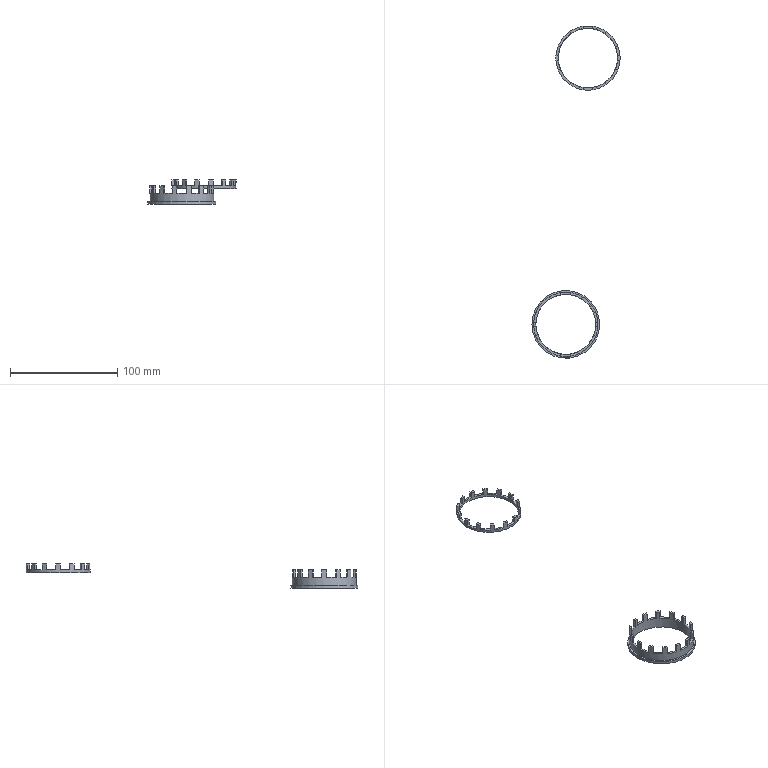CAM job | NX | 3-axis milling | part box 82.344 x 310.506 x 22.5 mm | stock box 92.344 x 320.506 x 22.5 mm
Tools:
number,name,description,diameter,corner_radius,flute_length,length,flutes
6,D6,Milling Tool-5 Parameters,6.0,0.0,50.0,75.0,2
2,D2A45,Milling Tool-5 Parameters,2.0,0.0,50.0,75.0,2
Operations:
program,operation,operation_type,tool,method,geometry_group,spindle_rpm,surface_speed,feed_per_tooth,feed_cut,feed_plunge,cut_length_mm,path_length_mm,cut_time_min,machine_time_min
1,ZLEVEL_PROFILE_COPY_13,ZLevelMilling,D6,METHOD,A,9500.0,179.0,0.1158,2200.0,1000.0,445.421,542.266,0.2236,0.2333
1,ZLEVEL_PROFILE_COPY_13_COPY,ZLevelMilling,D6,METHOD,A,9500.0,179.0,0.1158,2200.0,1000.0,445.421,542.266,0.2236,0.2333
1,ZLEVEL_PROFILE_COPY_13_COPY_1,ZLevelMilling,D6,METHOD,A,9500.0,179.0,0.1158,2200.0,1000.0,445.421,542.266,0.2236,0.2333
1,ZLEVEL_PROFILE_COPY_13_COPY_2,ZLevelMilling,D6,METHOD,A,9500.0,179.0,0.1158,2200.0,1000.0,445.421,542.266,0.2236,0.2333
1,ZLEVEL_PROFILE_COPY_13_COPY_3,ZLevelMilling,D6,METHOD,A,9500.0,179.0,0.1158,2200.0,1000.0,445.421,542.266,0.2236,0.2333
1,ZLEVEL_PROFILE_COPY_13_COPY_4,ZLevelMilling,D6,METHOD,A,9500.0,179.0,0.1158,2200.0,1000.0,445.421,542.266,0.2236,0.2333
1,ZLEVEL_PROFILE_COPY_13_COPY_5,ZLevelMilling,D6,METHOD,A,9500.0,179.0,0.1158,2200.0,1000.0,445.421,542.266,0.2236,0.2333
1,ZLEVEL_PROFILE_COPY_13_COPY_6,ZLevelMilling,D6,METHOD,A,9500.0,179.0,0.1158,2200.0,1000.0,445.421,542.266,0.2236,0.2333
1,ZLEVEL_PROFILE_COPY_13_COPY_7,ZLevelMilling,D6,METHOD,A,9500.0,179.0,0.1158,2200.0,1000.0,445.421,542.266,0.2236,0.2333
1,ZLEVEL_PROFILE_COPY_13_COPY_8,ZLevelMilling,D6,METHOD,A,9500.0,179.0,0.1158,2200.0,1000.0,445.421,542.266,0.2236,0.2333
1,ZLEVEL_PROFILE_COPY_13_COPY_9,ZLevelMilling,D6,METHOD,A,9500.0,179.0,0.1158,2200.0,1000.0,445.421,542.266,0.2236,0.2333
1,ZLEVEL_PROFILE_COPY_13_COPY_10,ZLevelMilling,D6,METHOD,A,9500.0,179.0,0.1158,2200.0,1000.0,445.421,542.266,0.2236,0.2333
1,ZLEVEL_PROFILE_COPY_13_COPY_11,ZLevelMilling,D6,METHOD,A,9500.0,179.0,0.1158,2200.0,1000.0,445.421,542.266,0.2236,0.2333
1,ZLEVEL_PROFILE_COPY_13_COPY_12,ZLevelMilling,D6,METHOD,A,9500.0,179.0,0.1158,2200.0,1000.0,445.421,542.266,0.2236,0.2333
1,PLANAR_MILL_1_COPY_13,PlanarMilling,D2A45,METHOD,A,9500.0,59.0,0.0658,1250.0,100.0,264.823,2396.501,0.2119,0.425
11,ZLEVEL_PROFILE_COPY_13_COPY_13,ZLevelMilling,D6,METHOD,B,9500.0,179.0,0.1158,2200.0,1000.0,269.188,356.65,0.1356,0.1444
11,ZLEVEL_PROFILE_COPY_13_COPY_13_COPY,ZLevelMilling,D6,METHOD,B,9500.0,179.0,0.1158,2200.0,1000.0,269.188,356.65,0.1356,0.1444
11,ZLEVEL_PROFILE_COPY_13_COPY_13_COPY_1,ZLevelMilling,D6,METHOD,B,9500.0,179.0,0.1158,2200.0,1000.0,269.188,356.65,0.1356,0.1444
11,ZLEVEL_PROFILE_COPY_13_COPY_13_COPY_2,ZLevelMilling,D6,METHOD,B,9500.0,179.0,0.1158,2200.0,1000.0,269.188,356.65,0.1356,0.1444
11,ZLEVEL_PROFILE_COPY_13_COPY_13_COPY_3,ZLevelMilling,D6,METHOD,B,9500.0,179.0,0.1158,2200.0,1000.0,269.188,356.65,0.1356,0.1444
11,ZLEVEL_PROFILE_COPY_13_COPY_13_COPY_4,ZLevelMilling,D6,METHOD,B,9500.0,179.0,0.1158,2200.0,1000.0,269.188,356.65,0.1356,0.1444
11,ZLEVEL_PROFILE_COPY_13_COPY_13_COPY_5,ZLevelMilling,D6,METHOD,B,9500.0,179.0,0.1158,2200.0,1000.0,269.188,356.65,0.1356,0.1444
11,ZLEVEL_PROFILE_COPY_13_COPY_13_COPY_6,ZLevelMilling,D6,METHOD,B,9500.0,179.0,0.1158,2200.0,1000.0,269.188,356.65,0.1356,0.1444
11,ZLEVEL_PROFILE_COPY_13_COPY_13_COPY_7,ZLevelMilling,D6,METHOD,B,9500.0,179.0,0.1158,2200.0,1000.0,269.188,356.65,0.1356,0.1444
11,ZLEVEL_PROFILE_COPY_13_COPY_13_COPY_8,ZLevelMilling,D6,METHOD,B,9500.0,179.0,0.1158,2200.0,1000.0,269.188,356.65,0.1356,0.1444
11,ZLEVEL_PROFILE_COPY_13_COPY_13_COPY_9,ZLevelMilling,D6,METHOD,B,9500.0,179.0,0.1158,2200.0,1000.0,269.188,356.65,0.1356,0.1444
11,ZLEVEL_PROFILE_COPY_13_COPY_13_COPY_10,ZLevelMilling,D6,METHOD,B,9500.0,179.0,0.1158,2200.0,1000.0,269.188,356.65,0.1356,0.1444
11,ZLEVEL_PROFILE_COPY_13_COPY_13_COPY_11,ZLevelMilling,D6,METHOD,B,9500.0,179.0,0.1158,2200.0,1000.0,269.188,356.65,0.1356,0.1444
11,ZLEVEL_PROFILE_COPY_13_COPY_13_COPY_12,ZLevelMilling,D6,METHOD,B,9500.0,179.0,0.1158,2200.0,1000.0,269.188,356.65,0.1356,0.1444
11,PLANAR_MILL,PlanarMilling,D6,METHOD,B,9500.0,179.0,0.0658,1250.0,100.0,27.765,333.257,0.0222,0.0528
11,PLANAR_MILL_COPY,PlanarMilling,D6,METHOD,B,9500.0,179.0,0.0658,1250.0,100.0,27.765,333.257,0.0222,0.0528
11,PLANAR_MILL_COPY_1,PlanarMilling,D6,METHOD,B,9500.0,179.0,0.0658,1250.0,100.0,27.765,333.257,0.0222,0.0528
11,PLANAR_MILL_COPY_2,PlanarMilling,D6,METHOD,B,9500.0,179.0,0.0658,1250.0,100.0,27.765,333.257,0.0222,0.0528
11,PLANAR_MILL_COPY_3,PlanarMilling,D6,METHOD,B,9500.0,179.0,0.0658,1250.0,100.0,27.765,333.257,0.0222,0.0528
11,PLANAR_MILL_COPY_4,PlanarMilling,D6,METHOD,B,9500.0,179.0,0.0658,1250.0,100.0,27.765,333.257,0.0222,0.0528
11,PLANAR_MILL_COPY_5,PlanarMilling,D6,METHOD,B,9500.0,179.0,0.0658,1250.0,100.0,27.765,333.257,0.0222,0.0528
11,PLANAR_MILL_COPY_6,PlanarMilling,D6,METHOD,B,9500.0,179.0,0.0658,1250.0,100.0,27.765,333.257,0.0222,0.0528
11,PLANAR_MILL_COPY_7,PlanarMilling,D6,METHOD,B,9500.0,179.0,0.0658,1250.0,100.0,27.765,333.257,0.0222,0.0528
11,PLANAR_MILL_COPY_8,PlanarMilling,D6,METHOD,B,9500.0,179.0,0.0658,1250.0,100.0,27.765,333.257,0.0222,0.0528
11,PLANAR_MILL_COPY_9,PlanarMilling,D6,METHOD,B,9500.0,179.0,0.0658,1250.0,100.0,27.765,333.257,0.0222,0.0528
11,PLANAR_MILL_COPY_10,PlanarMilling,D6,METHOD,B,9500.0,179.0,0.0658,1250.0,100.0,27.765,333.257,0.0222,0.0528
11,PLANAR_MILL_COPY_11,PlanarMilling,D6,METHOD,B,9500.0,179.0,0.0658,1250.0,100.0,27.765,333.257,0.0222,0.0528
11,PLANAR_MILL_COPY_12,PlanarMilling,D6,METHOD,B,9500.0,179.0,0.0658,1250.0,100.0,27.765,333.257,0.0222,0.0528
11,PLANAR_MILL_1,PlanarMilling,D2A45,METHOD,B,9500.0,59.0,0.0658,1250.0,100.0,19.055,168.844,0.0152,0.0302
11,PLANAR_MILL_1_COPY,PlanarMilling,D2A45,METHOD,B,9500.0,59.0,0.0658,1250.0,100.0,19.055,168.844,0.0152,0.0302
11,PLANAR_MILL_1_COPY_1,PlanarMilling,D2A45,METHOD,B,9500.0,59.0,0.0658,1250.0,100.0,19.055,168.844,0.0152,0.0302
11,PLANAR_MILL_1_COPY_2,PlanarMilling,D2A45,METHOD,B,9500.0,59.0,0.0658,1250.0,100.0,19.055,168.844,0.0152,0.0302
11,PLANAR_MILL_1_COPY_3,PlanarMilling,D2A45,METHOD,B,9500.0,59.0,0.0658,1250.0,100.0,19.055,168.844,0.0152,0.0302
11,PLANAR_MILL_1_COPY_4,PlanarMilling,D2A45,METHOD,B,9500.0,59.0,0.0658,1250.0,100.0,19.055,168.844,0.0152,0.0302
11,PLANAR_MILL_1_COPY_5,PlanarMilling,D2A45,METHOD,B,9500.0,59.0,0.0658,1250.0,100.0,19.055,168.844,0.0152,0.0302
11,PLANAR_MILL_1_COPY_6,PlanarMilling,D2A45,METHOD,B,9500.0,59.0,0.0658,1250.0,100.0,19.055,168.844,0.0152,0.0302
11,PLANAR_MILL_1_COPY_7,PlanarMilling,D2A45,METHOD,B,9500.0,59.0,0.0658,1250.0,100.0,19.055,168.844,0.0152,0.0302
11,PLANAR_MILL_1_COPY_8,PlanarMilling,D2A45,METHOD,B,9500.0,59.0,0.0658,1250.0,100.0,19.055,168.844,0.0152,0.0302
11,PLANAR_MILL_1_COPY_9,PlanarMilling,D2A45,METHOD,B,9500.0,59.0,0.0658,1250.0,100.0,19.055,168.844,0.0152,0.0302
11,PLANAR_MILL_1_COPY_10,PlanarMilling,D2A45,METHOD,B,9500.0,59.0,0.0658,1250.0,100.0,19.055,168.844,0.0152,0.0302
11,PLANAR_MILL_1_COPY_11,PlanarMilling,D2A45,METHOD,B,9500.0,59.0,0.0658,1250.0,100.0,19.055,168.844,0.0152,0.0302
11,PLANAR_MILL_1_COPY_12,PlanarMilling,D2A45,METHOD,B,9500.0,59.0,0.0658,1250.0,100.0,19.055,168.844,0.0152,0.0302